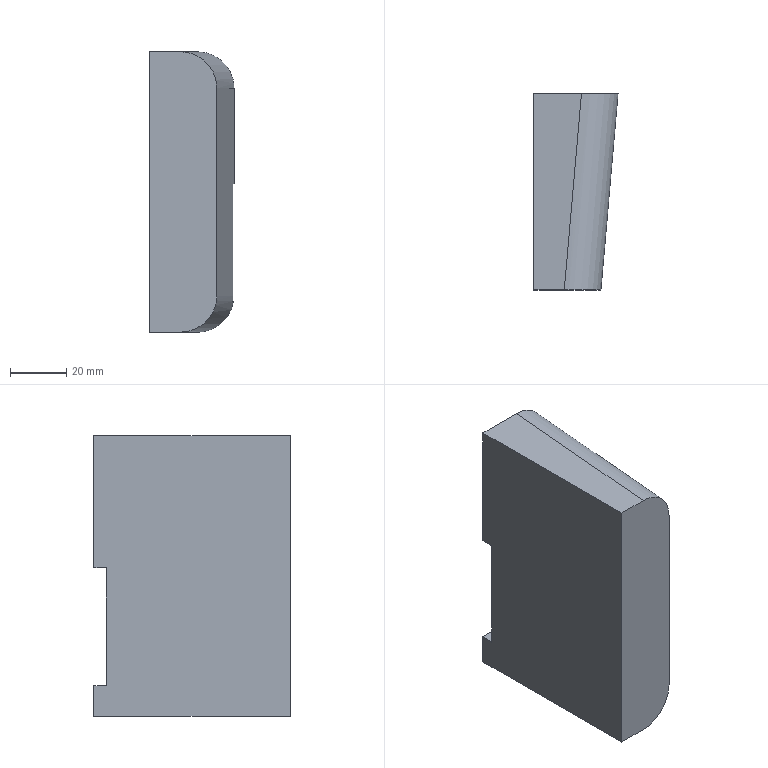Part | STEP file | 1 solid | 12 faces | box 30 x 70 x 100 mm | volume 177836 mm3 | plane 10 | cylinder 2 | commonest cylinder face diameters 26 x2
STEP:
#1=CARTESIAN_POINT('',(0.,0.,0.));
#2=DIRECTION('',(0.,0.,1.));
#3=DIRECTION('',(1.,0.,0.));
#4=AXIS2_PLACEMENT_3D('',#1,#2,#3);
#5=CARTESIAN_POINT('',(37.138,70.,139.451));
#6=VERTEX_POINT('',#5);
#7=CARTESIAN_POINT('',(66.97,70.,139.451));
#8=VERTEX_POINT('',#7);
#9=CARTESIAN_POINT('',(-72.862,70.,139.451));
#10=DIRECTION('',(1.,0.,0.));
#11=VECTOR('',#10,1.);
#12=LINE('',#9,#11);
#13=CARTESIAN_POINT('',(-72.862,70.,-363.47));
#14=DIRECTION('',(0.,-1.,0.));
#15=DIRECTION('',(0.,0.,-1.));
#16=AXIS2_PLACEMENT_3D('',#13,#14,#15);
#17=PLANE('',#16);
#18=CARTESIAN_POINT('',(-502.922,0.));
#19=DIRECTION('',(0.,1.));
#20=VECTOR('',#19,1.);
#21=LINE('',#18,#20);
#22=(GEOMETRIC_REPRESENTATION_CONTEXT(2)PARAMETRIC_REPRESENTATION_CONTEXT()REPRESENTATION_CONTEXT('',''));
#23=DEFINITIONAL_REPRESENTATION('',(#21),#22);
#24=PCURVE('',#17,#23);
#25=CARTESIAN_POINT('',(47.085,69.939,139.451));
#26=DIRECTION('',(0.,0.,1.));
#27=DIRECTION('',(-1.,0.,0.));
#28=AXIS2_PLACEMENT_3D('',#25,#26,#27);
#29=PLANE('',#28);
#30=CARTESIAN_POINT('',(119.948,-0.06099));
#31=DIRECTION('',(-1.,0.));
#32=VECTOR('',#31,1.);
#33=LINE('',#30,#32);
#34=(GEOMETRIC_REPRESENTATION_CONTEXT(2)PARAMETRIC_REPRESENTATION_CONTEXT()REPRESENTATION_CONTEXT('',''));
#35=DEFINITIONAL_REPRESENTATION('',(#33),#34);
#36=PCURVE('',#29,#35);
#37=SURFACE_CURVE('',#12,(#24,#36),.PCURVE_S1.);
#38=EDGE_CURVE('',#6,#8,#37,.T.);
#39=ORIENTED_EDGE('',*,*,#38,.T.);
#40=CARTESIAN_POINT('',(54.088,70.,128.53));
#41=VERTEX_POINT('',#40);
#42=CARTESIAN_POINT('',(66.97,70.,139.451));
#43=CARTESIAN_POINT('',(65.898,70.,132.858));
#44=CARTESIAN_POINT('',(60.792,70.,128.53));
#45=CARTESIAN_POINT('',(54.088,70.,128.53));
#46=(BOUNDED_CURVE()B_SPLINE_CURVE(3,(#42,#43,#44,#45),.UNSPECIFIED.,.F.,.F.)B_SPLINE_CURVE_WITH_KNOTS((4,4),(3.302,4.712),.PIECEWISE_BEZIER_KNOTS.)CURVE()GEOMETRIC_REPRESENTATION_ITEM()RATIONAL_B_SPLINE_CURVE((1.,0.841,0.841,1.))REPRESENTATION_ITEM(''));
#47=CARTESIAN_POINT('',(-502.922,139.832));
#48=CARTESIAN_POINT('',(-496.329,138.76));
#49=CARTESIAN_POINT('',(-492.,133.655));
#50=CARTESIAN_POINT('',(-492.,126.95));
#51=(BOUNDED_CURVE()B_SPLINE_CURVE(3,(#47,#48,#49,#50),.UNSPECIFIED.,.F.,.F.)B_SPLINE_CURVE_WITH_KNOTS((4,4),(3.302,4.712),.PIECEWISE_BEZIER_KNOTS.)CURVE()GEOMETRIC_REPRESENTATION_ITEM()RATIONAL_B_SPLINE_CURVE((1.,0.841,0.841,1.))REPRESENTATION_ITEM(''));
#52=(GEOMETRIC_REPRESENTATION_CONTEXT(2)PARAMETRIC_REPRESENTATION_CONTEXT()REPRESENTATION_CONTEXT('',''));
#53=DEFINITIONAL_REPRESENTATION('',(#51),#52);
#54=PCURVE('',#17,#53);
#55=CARTESIAN_POINT('',(61.057,149.657,141.53));
#56=DIRECTION('',(-0.08716,-0.9962,0.));
#57=DIRECTION('',(0.9962,-0.08716,0.));
#58=AXIS2_PLACEMENT_3D('',#55,#56,#57);
#59=CYLINDRICAL_SURFACE('',#58,13.);
#60=CARTESIAN_POINT('',(6.123,78.839));
#61=CARTESIAN_POINT('',(6.103,78.842));
#62=CARTESIAN_POINT('',(6.063,78.851));
#63=CARTESIAN_POINT('',(6.003,78.868));
#64=CARTESIAN_POINT('',(5.941,78.889));
#65=CARTESIAN_POINT('',(5.878,78.916));
#66=CARTESIAN_POINT('',(5.814,78.946));
#67=CARTESIAN_POINT('',(5.749,78.982));
#68=CARTESIAN_POINT('',(5.684,79.022));
#69=CARTESIAN_POINT('',(5.618,79.066));
#70=CARTESIAN_POINT('',(5.551,79.115));
#71=CARTESIAN_POINT('',(5.484,79.167));
#72=CARTESIAN_POINT('',(5.418,79.224));
#73=CARTESIAN_POINT('',(5.351,79.283));
#74=CARTESIAN_POINT('',(5.284,79.346));
#75=CARTESIAN_POINT('',(5.217,79.411));
#76=CARTESIAN_POINT('',(5.151,79.478));
#77=CARTESIAN_POINT('',(5.086,79.546));
#78=CARTESIAN_POINT('',(5.021,79.615));
#79=CARTESIAN_POINT('',(4.957,79.685));
#80=CARTESIAN_POINT('',(4.894,79.755));
#81=CARTESIAN_POINT('',(4.833,79.825));
#82=CARTESIAN_POINT('',(4.772,79.894));
#83=CARTESIAN_POINT('',(4.732,79.939));
#84=CARTESIAN_POINT('',(4.712,79.961));
#85=B_SPLINE_CURVE_WITH_KNOTS('',3,(#60,#61,#62,#63,#64,#65,#66,#67,#68,#69,#70,#71,#72,#73,#74,#75,#76,#77,#78,#79,#80,#81,#82,#83,#84),.UNSPECIFIED.,.F.,.F.,(4,1,1,1,1,1,1,1,1,1,1,1,1,1,1,1,1,1,1,1,1,1,4),(3.302,3.366,3.43,3.494,3.559,3.623,3.687,3.751,3.815,3.879,3.943,4.007,4.071,4.135,4.2,4.264,4.328,4.392,4.456,4.52,4.584,4.648,4.712),.QUASI_UNIFORM_KNOTS.);
#86=(GEOMETRIC_REPRESENTATION_CONTEXT(2)PARAMETRIC_REPRESENTATION_CONTEXT()REPRESENTATION_CONTEXT('',''));
#87=DEFINITIONAL_REPRESENTATION('',(#85),#86);
#88=PCURVE('',#59,#87);
#89=SURFACE_CURVE('',#46,(#54,#88),.PCURVE_S1.);
#90=EDGE_CURVE('',#8,#41,#89,.T.);
#91=ORIENTED_EDGE('',*,*,#90,.T.);
#92=CARTESIAN_POINT('',(37.138,70.,128.53));
#93=VERTEX_POINT('',#92);
#94=CARTESIAN_POINT('',(57.138,70.,128.53));
#95=DIRECTION('',(-1.,0.,0.));
#96=VECTOR('',#95,1.);
#97=LINE('',#94,#96);
#98=CARTESIAN_POINT('',(-492.,130.));
#99=DIRECTION('',(0.,-1.));
#100=VECTOR('',#99,1.);
#101=LINE('',#98,#100);
#102=(GEOMETRIC_REPRESENTATION_CONTEXT(2)PARAMETRIC_REPRESENTATION_CONTEXT()REPRESENTATION_CONTEXT('',''));
#103=DEFINITIONAL_REPRESENTATION('',(#101),#102);
#104=PCURVE('',#17,#103);
#105=CARTESIAN_POINT('',(57.138,150.,128.53));
#106=DIRECTION('',(0.,0.,1.));
#107=DIRECTION('',(1.,0.,0.));
#108=AXIS2_PLACEMENT_3D('',#105,#106,#107);
#109=PLANE('',#108);
#110=CARTESIAN_POINT('',(0.,-80.));
#111=DIRECTION('',(-1.,0.));
#112=VECTOR('',#111,1.);
#113=LINE('',#110,#112);
#114=(GEOMETRIC_REPRESENTATION_CONTEXT(2)PARAMETRIC_REPRESENTATION_CONTEXT()REPRESENTATION_CONTEXT('',''));
#115=DEFINITIONAL_REPRESENTATION('',(#113),#114);
#116=PCURVE('',#109,#115);
#117=SURFACE_CURVE('',#97,(#104,#116),.PCURVE_S1.);
#118=EDGE_CURVE('',#41,#93,#117,.T.);
#119=ORIENTED_EDGE('',*,*,#118,.T.);
#120=CARTESIAN_POINT('',(37.138,70.,128.53));
#121=DIRECTION('',(0.,0.,1.));
#122=VECTOR('',#121,1.);
#123=LINE('',#120,#122);
#124=CARTESIAN_POINT('',(-492.,110.));
#125=DIRECTION('',(-1.,0.));
#126=VECTOR('',#125,1.);
#127=LINE('',#124,#126);
#128=(GEOMETRIC_REPRESENTATION_CONTEXT(2)PARAMETRIC_REPRESENTATION_CONTEXT()REPRESENTATION_CONTEXT('',''));
#129=DEFINITIONAL_REPRESENTATION('',(#127),#128);
#130=PCURVE('',#17,#129);
#131=CARTESIAN_POINT('',(37.138,150.,128.53));
#132=DIRECTION('',(1.,0.,0.));
#133=DIRECTION('',(0.,0.,-1.));
#134=AXIS2_PLACEMENT_3D('',#131,#132,#133);
#135=PLANE('',#134);
#136=CARTESIAN_POINT('',(0.,-80.));
#137=DIRECTION('',(-1.,0.));
#138=VECTOR('',#137,1.);
#139=LINE('',#136,#138);
#140=(GEOMETRIC_REPRESENTATION_CONTEXT(2)PARAMETRIC_REPRESENTATION_CONTEXT()REPRESENTATION_CONTEXT('',''));
#141=DEFINITIONAL_REPRESENTATION('',(#139),#140);
#142=PCURVE('',#135,#141);
#143=SURFACE_CURVE('',#123,(#130,#142),.PCURVE_S1.);
#144=EDGE_CURVE('',#93,#6,#143,.T.);
#145=ORIENTED_EDGE('',*,*,#144,.T.);
#146=EDGE_LOOP('',(#39,#91,#119,#145));
#147=FACE_BOUND('',#146,.T.);
#148=ADVANCED_FACE('',(#147),#17,.F.);
#149=ORIENTED_EDGE('',*,*,#90,.F.);
#150=CARTESIAN_POINT('',(66.576,65.5,139.451));
#151=VERTEX_POINT('',#150);
#152=CARTESIAN_POINT('',(66.774,67.761,139.451));
#153=DIRECTION('',(-0.08716,-0.9962,0.));
#154=VECTOR('',#153,1.);
#155=LINE('',#152,#154);
#156=CARTESIAN_POINT('',(6.123,81.087));
#157=DIRECTION('',(0.,1.));
#158=VECTOR('',#157,1.);
#159=LINE('',#156,#158);
#160=(GEOMETRIC_REPRESENTATION_CONTEXT(2)PARAMETRIC_REPRESENTATION_CONTEXT()REPRESENTATION_CONTEXT('',''));
#161=DEFINITIONAL_REPRESENTATION('',(#159),#160);
#162=PCURVE('',#59,#161);
#163=CARTESIAN_POINT('',(-19.688,2.178));
#164=DIRECTION('',(0.08716,0.9962));
#165=VECTOR('',#164,1.);
#166=LINE('',#163,#165);
#167=(GEOMETRIC_REPRESENTATION_CONTEXT(2)PARAMETRIC_REPRESENTATION_CONTEXT()REPRESENTATION_CONTEXT('',''));
#168=DEFINITIONAL_REPRESENTATION('',(#166),#167);
#169=PCURVE('',#29,#168);
#170=SURFACE_CURVE('',#155,(#162,#169),.PCURVE_S1.);
#171=EDGE_CURVE('',#8,#151,#170,.T.);
#172=ORIENTED_EDGE('',*,*,#171,.T.);
#173=CARTESIAN_POINT('',(66.744,65.5,141.53));
#174=VERTEX_POINT('',#173);
#175=CARTESIAN_POINT('',(66.576,65.5,139.451));
#176=CARTESIAN_POINT('',(66.688,65.5,140.139));
#177=CARTESIAN_POINT('',(66.744,65.5,140.833));
#178=CARTESIAN_POINT('',(66.744,65.5,141.53));
#179=(BOUNDED_CURVE()B_SPLINE_CURVE(3,(#175,#176,#177,#178),.UNSPECIFIED.,.F.,.F.)B_SPLINE_CURVE_WITH_KNOTS((4,4),(2.981,3.142),.PIECEWISE_BEZIER_KNOTS.)CURVE()GEOMETRIC_REPRESENTATION_ITEM()RATIONAL_B_SPLINE_CURVE((1.,0.9979,0.9979,1.))REPRESENTATION_ITEM(''));
#180=CARTESIAN_POINT('',(6.123,83.356));
#181=CARTESIAN_POINT('',(6.125,83.355));
#182=CARTESIAN_POINT('',(6.13,83.355));
#183=CARTESIAN_POINT('',(6.137,83.353));
#184=CARTESIAN_POINT('',(6.145,83.352));
#185=CARTESIAN_POINT('',(6.152,83.351));
#186=CARTESIAN_POINT('',(6.159,83.35));
#187=CARTESIAN_POINT('',(6.166,83.349));
#188=CARTESIAN_POINT('',(6.174,83.348));
#189=CARTESIAN_POINT('',(6.181,83.347));
#190=CARTESIAN_POINT('',(6.188,83.346));
#191=CARTESIAN_POINT('',(6.196,83.346));
#192=CARTESIAN_POINT('',(6.203,83.345));
#193=CARTESIAN_POINT('',(6.21,83.344));
#194=CARTESIAN_POINT('',(6.218,83.344));
#195=CARTESIAN_POINT('',(6.225,83.343));
#196=CARTESIAN_POINT('',(6.232,83.343));
#197=CARTESIAN_POINT('',(6.239,83.342));
#198=CARTESIAN_POINT('',(6.247,83.342));
#199=CARTESIAN_POINT('',(6.254,83.342));
#200=CARTESIAN_POINT('',(6.261,83.341));
#201=CARTESIAN_POINT('',(6.269,83.341));
#202=CARTESIAN_POINT('',(6.276,83.341));
#203=CARTESIAN_POINT('',(6.281,83.341));
#204=CARTESIAN_POINT('',(6.283,83.341));
#205=B_SPLINE_CURVE_WITH_KNOTS('',3,(#180,#181,#182,#183,#184,#185,#186,#187,#188,#189,#190,#191,#192,#193,#194,#195,#196,#197,#198,#199,#200,#201,#202,#203,#204),.UNSPECIFIED.,.F.,.F.,(4,1,1,1,1,1,1,1,1,1,1,1,1,1,1,1,1,1,1,1,1,1,4),(2.981,2.988,2.996,3.003,3.01,3.018,3.025,3.032,3.039,3.047,3.054,3.061,3.069,3.076,3.083,3.091,3.098,3.105,3.112,3.12,3.127,3.134,3.142),.QUASI_UNIFORM_KNOTS.);
#206=(GEOMETRIC_REPRESENTATION_CONTEXT(2)PARAMETRIC_REPRESENTATION_CONTEXT()REPRESENTATION_CONTEXT('',''));
#207=DEFINITIONAL_REPRESENTATION('',(#205),#206);
#208=PCURVE('',#59,#207);
#209=CARTESIAN_POINT('',(62.138,65.5,160.451));
#210=DIRECTION('',(0.,1.,0.));
#211=DIRECTION('',(0.,0.,1.));
#212=AXIS2_PLACEMENT_3D('',#209,#210,#211);
#213=PLANE('',#212);
#214=CARTESIAN_POINT('',(-21.,4.438));
#215=CARTESIAN_POINT('',(-20.312,4.55));
#216=CARTESIAN_POINT('',(-19.618,4.606));
#217=CARTESIAN_POINT('',(-18.922,4.606));
#218=(BOUNDED_CURVE()B_SPLINE_CURVE(3,(#214,#215,#216,#217),.UNSPECIFIED.,.F.,.F.)B_SPLINE_CURVE_WITH_KNOTS((4,4),(2.981,3.142),.PIECEWISE_BEZIER_KNOTS.)CURVE()GEOMETRIC_REPRESENTATION_ITEM()RATIONAL_B_SPLINE_CURVE((1.,0.9979,0.9979,1.))REPRESENTATION_ITEM(''));
#219=(GEOMETRIC_REPRESENTATION_CONTEXT(2)PARAMETRIC_REPRESENTATION_CONTEXT()REPRESENTATION_CONTEXT('',''));
#220=DEFINITIONAL_REPRESENTATION('',(#218),#219);
#221=PCURVE('',#213,#220);
#222=SURFACE_CURVE('',#179,(#208,#221),.PCURVE_S1.);
#223=EDGE_CURVE('',#151,#174,#222,.T.);
#224=ORIENTED_EDGE('',*,*,#223,.T.);
#225=CARTESIAN_POINT('',(61.013,0.,141.53));
#226=VERTEX_POINT('',#225);
#227=CARTESIAN_POINT('',(67.138,70.,141.53));
#228=DIRECTION('',(0.08716,0.9962,0.));
#229=VECTOR('',#228,1.);
#230=LINE('',#227,#229);
#231=CARTESIAN_POINT('',(6.283,78.824));
#232=DIRECTION('',(0.,-1.));
#233=VECTOR('',#232,1.);
#234=LINE('',#231,#233);
#235=(GEOMETRIC_REPRESENTATION_CONTEXT(2)PARAMETRIC_REPRESENTATION_CONTEXT()REPRESENTATION_CONTEXT('',''));
#236=DEFINITIONAL_REPRESENTATION('',(#234),#235);
#237=PCURVE('',#59,#236);
#238=CARTESIAN_POINT('',(67.138,70.,178.53));
#239=DIRECTION('',(-0.9962,0.08716,0.));
#240=DIRECTION('',(-0.08716,-0.9962,0.));
#241=AXIS2_PLACEMENT_3D('',#238,#239,#240);
#242=PLANE('',#241);
#243=CARTESIAN_POINT('',(0.,-37.));
#244=DIRECTION('',(-1.,0.));
#245=VECTOR('',#244,1.);
#246=LINE('',#243,#245);
#247=(GEOMETRIC_REPRESENTATION_CONTEXT(2)PARAMETRIC_REPRESENTATION_CONTEXT()REPRESENTATION_CONTEXT('',''));
#248=DEFINITIONAL_REPRESENTATION('',(#246),#247);
#249=PCURVE('',#242,#248);
#250=SURFACE_CURVE('',#230,(#237,#249),.PCURVE_S1.);
#251=EDGE_CURVE('',#226,#174,#250,.T.);
#252=ORIENTED_EDGE('',*,*,#251,.F.);
#253=CARTESIAN_POINT('',(47.964,0.,128.53));
#254=VERTEX_POINT('',#253);
#255=CARTESIAN_POINT('',(47.964,0.,128.53));
#256=CARTESIAN_POINT('',(55.608,0.,128.53));
#257=CARTESIAN_POINT('',(61.013,0.,133.914));
#258=CARTESIAN_POINT('',(61.013,0.,141.53));
#259=(BOUNDED_CURVE()B_SPLINE_CURVE(3,(#255,#256,#257,#258),.UNSPECIFIED.,.F.,.F.)B_SPLINE_CURVE_WITH_KNOTS((4,4),(1.571,3.142),.PIECEWISE_BEZIER_KNOTS.)CURVE()GEOMETRIC_REPRESENTATION_ITEM()RATIONAL_B_SPLINE_CURVE((1.,0.8047,0.8047,1.))REPRESENTATION_ITEM(''));
#260=CARTESIAN_POINT('',(4.712,150.229));
#261=CARTESIAN_POINT('',(4.734,150.204));
#262=CARTESIAN_POINT('',(4.777,150.155));
#263=CARTESIAN_POINT('',(4.844,150.079));
#264=CARTESIAN_POINT('',(4.912,150.003));
#265=CARTESIAN_POINT('',(4.982,149.925));
#266=CARTESIAN_POINT('',(5.053,149.848));
#267=CARTESIAN_POINT('',(5.125,149.772));
#268=CARTESIAN_POINT('',(5.199,149.697));
#269=CARTESIAN_POINT('',(5.273,149.624));
#270=CARTESIAN_POINT('',(5.347,149.553));
#271=CARTESIAN_POINT('',(5.422,149.487));
#272=CARTESIAN_POINT('',(5.498,149.424));
#273=CARTESIAN_POINT('',(5.573,149.365));
#274=CARTESIAN_POINT('',(5.648,149.312));
#275=CARTESIAN_POINT('',(5.723,149.264));
#276=CARTESIAN_POINT('',(5.797,149.222));
#277=CARTESIAN_POINT('',(5.87,149.186));
#278=CARTESIAN_POINT('',(5.942,149.156));
#279=CARTESIAN_POINT('',(6.013,149.132));
#280=CARTESIAN_POINT('',(6.083,149.113));
#281=CARTESIAN_POINT('',(6.152,149.1));
#282=CARTESIAN_POINT('',(6.218,149.093));
#283=CARTESIAN_POINT('',(6.262,149.091));
#284=CARTESIAN_POINT('',(6.283,149.091));
#285=B_SPLINE_CURVE_WITH_KNOTS('',3,(#260,#261,#262,#263,#264,#265,#266,#267,#268,#269,#270,#271,#272,#273,#274,#275,#276,#277,#278,#279,#280,#281,#282,#283,#284),.UNSPECIFIED.,.F.,.F.,(4,1,1,1,1,1,1,1,1,1,1,1,1,1,1,1,1,1,1,1,1,1,4),(1.571,1.642,1.714,1.785,1.856,1.928,1.999,2.071,2.142,2.213,2.285,2.356,2.428,2.499,2.57,2.642,2.713,2.785,2.856,2.927,2.999,3.07,3.142),.QUASI_UNIFORM_KNOTS.);
#286=(GEOMETRIC_REPRESENTATION_CONTEXT(2)PARAMETRIC_REPRESENTATION_CONTEXT()REPRESENTATION_CONTEXT('',''));
#287=DEFINITIONAL_REPRESENTATION('',(#285),#286);
#288=PCURVE('',#59,#287);
#289=CARTESIAN_POINT('',(52.138,0.,178.53));
#290=DIRECTION('',(0.,1.,0.));
#291=DIRECTION('',(0.,0.,1.));
#292=AXIS2_PLACEMENT_3D('',#289,#290,#291);
#293=PLANE('',#292);
#294=CARTESIAN_POINT('',(-50.,-4.174));
#295=CARTESIAN_POINT('',(-50.,3.47));
#296=CARTESIAN_POINT('',(-44.615,8.876));
#297=CARTESIAN_POINT('',(-37.,8.876));
#298=(BOUNDED_CURVE()B_SPLINE_CURVE(3,(#294,#295,#296,#297),.UNSPECIFIED.,.F.,.F.)B_SPLINE_CURVE_WITH_KNOTS((4,4),(1.571,3.142),.PIECEWISE_BEZIER_KNOTS.)CURVE()GEOMETRIC_REPRESENTATION_ITEM()RATIONAL_B_SPLINE_CURVE((1.,0.8047,0.8047,1.))REPRESENTATION_ITEM(''));
#299=(GEOMETRIC_REPRESENTATION_CONTEXT(2)PARAMETRIC_REPRESENTATION_CONTEXT()REPRESENTATION_CONTEXT('',''));
#300=DEFINITIONAL_REPRESENTATION('',(#298),#299);
#301=PCURVE('',#293,#300);
#302=SURFACE_CURVE('',#259,(#288,#301),.PCURVE_S1.);
#303=EDGE_CURVE('',#254,#226,#302,.T.);
#304=ORIENTED_EDGE('',*,*,#303,.F.);
#305=CARTESIAN_POINT('',(61.057,149.657,128.53));
#306=DIRECTION('',(-0.08716,-0.9962,0.));
#307=VECTOR('',#306,1.);
#308=LINE('',#305,#307);
#309=CARTESIAN_POINT('',(4.712,0.));
#310=DIRECTION('',(0.,1.));
#311=VECTOR('',#310,1.);
#312=LINE('',#309,#311);
#313=(GEOMETRIC_REPRESENTATION_CONTEXT(2)PARAMETRIC_REPRESENTATION_CONTEXT()REPRESENTATION_CONTEXT('',''));
#314=DEFINITIONAL_REPRESENTATION('',(#312),#313);
#315=PCURVE('',#59,#314);
#316=CARTESIAN_POINT('',(3.919,-0.3429));
#317=DIRECTION('',(-0.08716,-0.9962));
#318=VECTOR('',#317,1.);
#319=LINE('',#316,#318);
#320=(GEOMETRIC_REPRESENTATION_CONTEXT(2)PARAMETRIC_REPRESENTATION_CONTEXT()REPRESENTATION_CONTEXT('',''));
#321=DEFINITIONAL_REPRESENTATION('',(#319),#320);
#322=PCURVE('',#109,#321);
#323=SURFACE_CURVE('',#308,(#315,#322),.PCURVE_S1.);
#324=EDGE_CURVE('',#41,#254,#323,.T.);
#325=ORIENTED_EDGE('',*,*,#324,.F.);
#326=EDGE_LOOP('',(#149,#172,#224,#252,#304,#325));
#327=FACE_BOUND('',#326,.T.);
#328=ADVANCED_FACE('',(#327),#59,.T.);
#329=CARTESIAN_POINT('',(37.138,65.5,181.451));
#330=VERTEX_POINT('',#329);
#331=CARTESIAN_POINT('',(37.138,65.5,139.451));
#332=VERTEX_POINT('',#331);
#333=CARTESIAN_POINT('',(37.138,65.5,108.53));
#334=DIRECTION('',(0.,0.,-1.));
#335=VECTOR('',#334,1.);
#336=LINE('',#333,#335);
#337=CARTESIAN_POINT('',(20.,-84.5));
#338=DIRECTION('',(1.,0.));
#339=VECTOR('',#338,1.);
#340=LINE('',#337,#339);
#341=(GEOMETRIC_REPRESENTATION_CONTEXT(2)PARAMETRIC_REPRESENTATION_CONTEXT()REPRESENTATION_CONTEXT('',''));
#342=DEFINITIONAL_REPRESENTATION('',(#340),#341);
#343=PCURVE('',#135,#342);
#344=CARTESIAN_POINT('',(-51.922,-25.));
#345=DIRECTION('',(-1.,0.));
#346=VECTOR('',#345,1.);
#347=LINE('',#344,#346);
#348=(GEOMETRIC_REPRESENTATION_CONTEXT(2)PARAMETRIC_REPRESENTATION_CONTEXT()REPRESENTATION_CONTEXT('',''));
#349=DEFINITIONAL_REPRESENTATION('',(#347),#348);
#350=PCURVE('',#213,#349);
#351=SURFACE_CURVE('',#336,(#343,#350),.PCURVE_S1.);
#352=EDGE_CURVE('',#330,#332,#351,.T.);
#353=ORIENTED_EDGE('',*,*,#352,.T.);
#354=CARTESIAN_POINT('',(37.138,69.939,139.451));
#355=DIRECTION('',(0.,1.,0.));
#356=VECTOR('',#355,1.);
#357=LINE('',#354,#356);
#358=CARTESIAN_POINT('',(-10.922,-80.061));
#359=DIRECTION('',(0.,1.));
#360=VECTOR('',#359,1.);
#361=LINE('',#358,#360);
#362=(GEOMETRIC_REPRESENTATION_CONTEXT(2)PARAMETRIC_REPRESENTATION_CONTEXT()REPRESENTATION_CONTEXT('',''));
#363=DEFINITIONAL_REPRESENTATION('',(#361),#362);
#364=PCURVE('',#135,#363);
#365=CARTESIAN_POINT('',(9.948,0.));
#366=DIRECTION('',(0.,-1.));
#367=VECTOR('',#366,1.);
#368=LINE('',#365,#367);
#369=(GEOMETRIC_REPRESENTATION_CONTEXT(2)PARAMETRIC_REPRESENTATION_CONTEXT()REPRESENTATION_CONTEXT('',''));
#370=DEFINITIONAL_REPRESENTATION('',(#368),#369);
#371=PCURVE('',#29,#370);
#372=SURFACE_CURVE('',#357,(#364,#371),.PCURVE_S1.);
#373=EDGE_CURVE('',#332,#6,#372,.T.);
#374=ORIENTED_EDGE('',*,*,#373,.T.);
#375=ORIENTED_EDGE('',*,*,#144,.F.);
#376=CARTESIAN_POINT('',(37.138,0.,128.53));
#377=VERTEX_POINT('',#376);
#378=CARTESIAN_POINT('',(37.138,150.,128.53));
#379=DIRECTION('',(0.,-1.,0.));
#380=VECTOR('',#379,1.);
#381=LINE('',#378,#380);
#382=CARTESIAN_POINT('',(0.,0.));
#383=DIRECTION('',(0.,-1.));
#384=VECTOR('',#383,1.);
#385=LINE('',#382,#384);
#386=(GEOMETRIC_REPRESENTATION_CONTEXT(2)PARAMETRIC_REPRESENTATION_CONTEXT()REPRESENTATION_CONTEXT('',''));
#387=DEFINITIONAL_REPRESENTATION('',(#385),#386);
#388=PCURVE('',#135,#387);
#389=CARTESIAN_POINT('',(-20.,0.));
#390=DIRECTION('',(0.,-1.));
#391=VECTOR('',#390,1.);
#392=LINE('',#389,#391);
#393=(GEOMETRIC_REPRESENTATION_CONTEXT(2)PARAMETRIC_REPRESENTATION_CONTEXT()REPRESENTATION_CONTEXT('',''));
#394=DEFINITIONAL_REPRESENTATION('',(#392),#393);
#395=PCURVE('',#109,#394);
#396=SURFACE_CURVE('',#381,(#388,#395),.PCURVE_S1.);
#397=EDGE_CURVE('',#93,#377,#396,.T.);
#398=ORIENTED_EDGE('',*,*,#397,.T.);
#399=CARTESIAN_POINT('',(37.138,0.,228.53));
#400=VERTEX_POINT('',#399);
#401=CARTESIAN_POINT('',(37.138,0.,128.53));
#402=DIRECTION('',(0.,0.,1.));
#403=VECTOR('',#402,1.);
#404=LINE('',#401,#403);
#405=CARTESIAN_POINT('',(0.,-150.));
#406=DIRECTION('',(-1.,0.));
#407=VECTOR('',#406,1.);
#408=LINE('',#405,#407);
#409=(GEOMETRIC_REPRESENTATION_CONTEXT(2)PARAMETRIC_REPRESENTATION_CONTEXT()REPRESENTATION_CONTEXT('',''));
#410=DEFINITIONAL_REPRESENTATION('',(#408),#409);
#411=PCURVE('',#135,#410);
#412=CARTESIAN_POINT('',(-50.,-15.));
#413=DIRECTION('',(1.,0.));
#414=VECTOR('',#413,1.);
#415=LINE('',#412,#414);
#416=(GEOMETRIC_REPRESENTATION_CONTEXT(2)PARAMETRIC_REPRESENTATION_CONTEXT()REPRESENTATION_CONTEXT('',''));
#417=DEFINITIONAL_REPRESENTATION('',(#415),#416);
#418=PCURVE('',#293,#417);
#419=SURFACE_CURVE('',#404,(#411,#418),.PCURVE_S1.);
#420=EDGE_CURVE('',#377,#400,#419,.T.);
#421=ORIENTED_EDGE('',*,*,#420,.T.);
#422=CARTESIAN_POINT('',(37.138,70.,228.53));
#423=VERTEX_POINT('',#422);
#424=CARTESIAN_POINT('',(37.138,150.,228.53));
#425=DIRECTION('',(0.,-1.,0.));
#426=VECTOR('',#425,1.);
#427=LINE('',#424,#426);
#428=CARTESIAN_POINT('',(-100.,0.));
#429=DIRECTION('',(0.,-1.));
#430=VECTOR('',#429,1.);
#431=LINE('',#428,#430);
#432=(GEOMETRIC_REPRESENTATION_CONTEXT(2)PARAMETRIC_REPRESENTATION_CONTEXT()REPRESENTATION_CONTEXT('',''));
#433=DEFINITIONAL_REPRESENTATION('',(#431),#432);
#434=PCURVE('',#135,#433);
#435=CARTESIAN_POINT('',(37.138,150.,228.53));
#436=DIRECTION('',(0.,0.,-1.));
#437=DIRECTION('',(-1.,0.,0.));
#438=AXIS2_PLACEMENT_3D('',#435,#436,#437);
#439=PLANE('',#438);
#440=CARTESIAN_POINT('',(0.,0.));
#441=DIRECTION('',(0.,-1.));
#442=VECTOR('',#441,1.);
#443=LINE('',#440,#442);
#444=(GEOMETRIC_REPRESENTATION_CONTEXT(2)PARAMETRIC_REPRESENTATION_CONTEXT()REPRESENTATION_CONTEXT('',''));
#445=DEFINITIONAL_REPRESENTATION('',(#443),#444);
#446=PCURVE('',#439,#445);
#447=SURFACE_CURVE('',#427,(#434,#446),.PCURVE_S1.);
#448=EDGE_CURVE('',#423,#400,#447,.T.);
#449=ORIENTED_EDGE('',*,*,#448,.F.);
#450=CARTESIAN_POINT('',(37.138,70.,181.451));
#451=VERTEX_POINT('',#450);
#452=CARTESIAN_POINT('',(37.138,70.,128.53));
#453=DIRECTION('',(0.,0.,1.));
#454=VECTOR('',#453,1.);
#455=LINE('',#452,#454);
#456=CARTESIAN_POINT('',(0.,-80.));
#457=DIRECTION('',(-1.,0.));
#458=VECTOR('',#457,1.);
#459=LINE('',#456,#458);
#460=(GEOMETRIC_REPRESENTATION_CONTEXT(2)PARAMETRIC_REPRESENTATION_CONTEXT()REPRESENTATION_CONTEXT('',''));
#461=DEFINITIONAL_REPRESENTATION('',(#459),#460);
#462=PCURVE('',#135,#461);
#463=CARTESIAN_POINT('',(-72.862,70.,-363.47));
#464=DIRECTION('',(0.,-1.,0.));
#465=DIRECTION('',(0.,0.,-1.));
#466=AXIS2_PLACEMENT_3D('',#463,#464,#465);
#467=PLANE('',#466);
#468=CARTESIAN_POINT('',(-492.,110.));
#469=DIRECTION('',(-1.,0.));
#470=VECTOR('',#469,1.);
#471=LINE('',#468,#470);
#472=(GEOMETRIC_REPRESENTATION_CONTEXT(2)PARAMETRIC_REPRESENTATION_CONTEXT()REPRESENTATION_CONTEXT('',''));
#473=DEFINITIONAL_REPRESENTATION('',(#471),#472);
#474=PCURVE('',#467,#473);
#475=SURFACE_CURVE('',#455,(#462,#474),.PCURVE_S1.);
#476=EDGE_CURVE('',#451,#423,#475,.T.);
#477=ORIENTED_EDGE('',*,*,#476,.F.);
#478=CARTESIAN_POINT('',(37.138,69.939,181.451));
#479=DIRECTION('',(0.,1.,0.));
#480=VECTOR('',#479,1.);
#481=LINE('',#478,#480);
#482=CARTESIAN_POINT('',(-52.922,-80.061));
#483=DIRECTION('',(0.,1.));
#484=VECTOR('',#483,1.);
#485=LINE('',#482,#484);
#486=(GEOMETRIC_REPRESENTATION_CONTEXT(2)PARAMETRIC_REPRESENTATION_CONTEXT()REPRESENTATION_CONTEXT('',''));
#487=DEFINITIONAL_REPRESENTATION('',(#485),#486);
#488=PCURVE('',#135,#487);
#489=CARTESIAN_POINT('',(47.085,69.939,181.451));
#490=DIRECTION('',(0.,0.,1.));
#491=DIRECTION('',(-1.,0.,0.));
#492=AXIS2_PLACEMENT_3D('',#489,#490,#491);
#493=PLANE('',#492);
#494=CARTESIAN_POINT('',(9.948,0.));
#495=DIRECTION('',(0.,-1.));
#496=VECTOR('',#495,1.);
#497=LINE('',#494,#496);
#498=(GEOMETRIC_REPRESENTATION_CONTEXT(2)PARAMETRIC_REPRESENTATION_CONTEXT()REPRESENTATION_CONTEXT('',''));
#499=DEFINITIONAL_REPRESENTATION('',(#497),#498);
#500=PCURVE('',#493,#499);
#501=SURFACE_CURVE('',#481,(#488,#500),.PCURVE_S1.);
#502=EDGE_CURVE('',#330,#451,#501,.T.);
#503=ORIENTED_EDGE('',*,*,#502,.F.);
#504=EDGE_LOOP('',(#353,#374,#375,#398,#421,#449,#477,#503));
#505=FACE_BOUND('',#504,.T.);
#506=ADVANCED_FACE('',(#505),#135,.F.);
#507=CARTESIAN_POINT('',(67.138,70.,215.53));
#508=VERTEX_POINT('',#507);
#509=CARTESIAN_POINT('',(67.138,70.,181.451));
#510=VERTEX_POINT('',#509);
#511=CARTESIAN_POINT('',(67.138,70.,178.53));
#512=DIRECTION('',(0.,0.,-1.));
#513=VECTOR('',#512,1.);
#514=LINE('',#511,#513);
#515=CARTESIAN_POINT('',(-542.,140.));
#516=DIRECTION('',(1.,0.));
#517=VECTOR('',#516,1.);
#518=LINE('',#515,#517);
#519=(GEOMETRIC_REPRESENTATION_CONTEXT(2)PARAMETRIC_REPRESENTATION_CONTEXT()REPRESENTATION_CONTEXT('',''));
#520=DEFINITIONAL_REPRESENTATION('',(#518),#519);
#521=PCURVE('',#467,#520);
#522=CARTESIAN_POINT('',(0.,0.));
#523=DIRECTION('',(0.,-1.));
#524=VECTOR('',#523,1.);
#525=LINE('',#522,#524);
#526=(GEOMETRIC_REPRESENTATION_CONTEXT(2)PARAMETRIC_REPRESENTATION_CONTEXT()REPRESENTATION_CONTEXT('',''));
#527=DEFINITIONAL_REPRESENTATION('',(#525),#526);
#528=PCURVE('',#242,#527);
#529=SURFACE_CURVE('',#514,(#521,#528),.PCURVE_S1.);
#530=EDGE_CURVE('',#508,#510,#529,.T.);
#531=ORIENTED_EDGE('',*,*,#530,.T.);
#532=CARTESIAN_POINT('',(-72.862,70.,181.451));
#533=DIRECTION('',(1.,0.,0.));
#534=VECTOR('',#533,1.);
#535=LINE('',#532,#534);
#536=CARTESIAN_POINT('',(-544.922,0.));
#537=DIRECTION('',(0.,1.));
#538=VECTOR('',#537,1.);
#539=LINE('',#536,#538);
#540=(GEOMETRIC_REPRESENTATION_CONTEXT(2)PARAMETRIC_REPRESENTATION_CONTEXT()REPRESENTATION_CONTEXT('',''));
#541=DEFINITIONAL_REPRESENTATION('',(#539),#540);
#542=PCURVE('',#467,#541);
#543=CARTESIAN_POINT('',(119.948,-0.06099));
#544=DIRECTION('',(-1.,0.));
#545=VECTOR('',#544,1.);
#546=LINE('',#543,#545);
#547=(GEOMETRIC_REPRESENTATION_CONTEXT(2)PARAMETRIC_REPRESENTATION_CONTEXT()REPRESENTATION_CONTEXT('',''));
#548=DEFINITIONAL_REPRESENTATION('',(#546),#547);
#549=PCURVE('',#493,#548);
#550=SURFACE_CURVE('',#535,(#542,#549),.PCURVE_S1.);
#551=EDGE_CURVE('',#451,#510,#550,.T.);
#552=ORIENTED_EDGE('',*,*,#551,.F.);
#553=ORIENTED_EDGE('',*,*,#476,.T.);
#554=CARTESIAN_POINT('',(54.088,70.,228.53));
#555=VERTEX_POINT('',#554);
#556=CARTESIAN_POINT('',(37.138,70.,228.53));
#557=DIRECTION('',(1.,0.,0.));
#558=VECTOR('',#557,1.);
#559=LINE('',#556,#558);
#560=CARTESIAN_POINT('',(-592.,110.));
#561=DIRECTION('',(0.,1.));
#562=VECTOR('',#561,1.);
#563=LINE('',#560,#562);
#564=(GEOMETRIC_REPRESENTATION_CONTEXT(2)PARAMETRIC_REPRESENTATION_CONTEXT()REPRESENTATION_CONTEXT('',''));
#565=DEFINITIONAL_REPRESENTATION('',(#563),#564);
#566=PCURVE('',#467,#565);
#567=CARTESIAN_POINT('',(0.,-80.));
#568=DIRECTION('',(-1.,0.));
#569=VECTOR('',#568,1.);
#570=LINE('',#567,#569);
#571=(GEOMETRIC_REPRESENTATION_CONTEXT(2)PARAMETRIC_REPRESENTATION_CONTEXT()REPRESENTATION_CONTEXT('',''));
#572=DEFINITIONAL_REPRESENTATION('',(#570),#571);
#573=PCURVE('',#439,#572);
#574=SURFACE_CURVE('',#559,(#566,#573),.PCURVE_S1.);
#575=EDGE_CURVE('',#423,#555,#574,.T.);
#576=ORIENTED_EDGE('',*,*,#575,.T.);
#577=CARTESIAN_POINT('',(54.088,70.,228.53));
#578=CARTESIAN_POINT('',(61.732,70.,228.53));
#579=CARTESIAN_POINT('',(67.138,70.,223.145));
#580=CARTESIAN_POINT('',(67.138,70.,215.53));
#581=(BOUNDED_CURVE()B_SPLINE_CURVE(3,(#577,#578,#579,#580),.UNSPECIFIED.,.F.,.F.)B_SPLINE_CURVE_WITH_KNOTS((4,4),(1.571,3.142),.PIECEWISE_BEZIER_KNOTS.)CURVE()GEOMETRIC_REPRESENTATION_ITEM()RATIONAL_B_SPLINE_CURVE((1.,0.8047,0.8047,1.))REPRESENTATION_ITEM(''));
#582=CARTESIAN_POINT('',(-592.,126.95));
#583=CARTESIAN_POINT('',(-592.,134.595));
#584=CARTESIAN_POINT('',(-586.615,140.));
#585=CARTESIAN_POINT('',(-579.,140.));
#586=(BOUNDED_CURVE()B_SPLINE_CURVE(3,(#582,#583,#584,#585),.UNSPECIFIED.,.F.,.F.)B_SPLINE_CURVE_WITH_KNOTS((4,4),(1.571,3.142),.PIECEWISE_BEZIER_KNOTS.)CURVE()GEOMETRIC_REPRESENTATION_ITEM()RATIONAL_B_SPLINE_CURVE((1.,0.8047,0.8047,1.))REPRESENTATION_ITEM(''));
#587=(GEOMETRIC_REPRESENTATION_CONTEXT(2)PARAMETRIC_REPRESENTATION_CONTEXT()REPRESENTATION_CONTEXT('',''));
#588=DEFINITIONAL_REPRESENTATION('',(#586),#587);
#589=PCURVE('',#467,#588);
#590=CARTESIAN_POINT('',(54.187,71.133,215.53));
#591=DIRECTION('',(-0.08716,-0.9962,0.));
#592=DIRECTION('',(0.9962,-0.08716,0.));
#593=AXIS2_PLACEMENT_3D('',#590,#591,#592);
#594=CYLINDRICAL_SURFACE('',#593,13.);
#595=CARTESIAN_POINT('',(1.571,1.137));
#596=CARTESIAN_POINT('',(1.549,1.113));
#597=CARTESIAN_POINT('',(1.506,1.064));
#598=CARTESIAN_POINT('',(1.439,0.988));
#599=CARTESIAN_POINT('',(1.371,0.9113));
#600=CARTESIAN_POINT('',(1.301,0.834));
#601=CARTESIAN_POINT('',(1.23,0.7569));
#602=CARTESIAN_POINT('',(1.158,0.6804));
#603=CARTESIAN_POINT('',(1.085,0.6054));
#604=CARTESIAN_POINT('',(1.01,0.5323));
#605=CARTESIAN_POINT('',(0.9358,0.4621));
#606=CARTESIAN_POINT('',(0.8607,0.3952));
#607=CARTESIAN_POINT('',(0.7854,0.3324));
#608=CARTESIAN_POINT('',(0.7101,0.2741));
#609=CARTESIAN_POINT('',(0.635,0.2208));
#610=CARTESIAN_POINT('',(0.5603,0.173));
#611=CARTESIAN_POINT('',(0.4863,0.1309));
#612=CARTESIAN_POINT('',(0.413,0.09472));
#613=CARTESIAN_POINT('',(0.3408,0.06449));
#614=CARTESIAN_POINT('',(0.2697,0.04021));
#615=CARTESIAN_POINT('',(0.2,0.02178));
#616=CARTESIAN_POINT('',(0.1316,0.008981));
#617=CARTESIAN_POINT('',(0.06485,0.001569));
#618=CARTESIAN_POINT('',(0.02143,-0.000003694));
#619=CARTESIAN_POINT('',(0.,0.));
#620=B_SPLINE_CURVE_WITH_KNOTS('',3,(#595,#596,#597,#598,#599,#600,#601,#602,#603,#604,#605,#606,#607,#608,#609,#610,#611,#612,#613,#614,#615,#616,#617,#618,#619),.UNSPECIFIED.,.F.,.F.,(4,1,1,1,1,1,1,1,1,1,1,1,1,1,1,1,1,1,1,1,1,1,4),(1.571,1.642,1.714,1.785,1.856,1.928,1.999,2.071,2.142,2.213,2.285,2.356,2.428,2.499,2.57,2.642,2.713,2.785,2.856,2.927,2.999,3.07,3.142),.QUASI_UNIFORM_KNOTS.);
#621=(GEOMETRIC_REPRESENTATION_CONTEXT(2)PARAMETRIC_REPRESENTATION_CONTEXT()REPRESENTATION_CONTEXT('',''));
#622=DEFINITIONAL_REPRESENTATION('',(#620),#621);
#623=PCURVE('',#594,#622);
#624=SURFACE_CURVE('',#581,(#589,#623),.PCURVE_S1.);
#625=EDGE_CURVE('',#555,#508,#624,.T.);
#626=ORIENTED_EDGE('',*,*,#625,.T.);
#627=EDGE_LOOP('',(#531,#552,#553,#576,#626));
#628=FACE_BOUND('',#627,.T.);
#629=ADVANCED_FACE('',(#628),#467,.F.);
#630=ORIENTED_EDGE('',*,*,#118,.F.);
#631=ORIENTED_EDGE('',*,*,#324,.T.);
#632=CARTESIAN_POINT('',(57.138,0.,128.53));
#633=DIRECTION('',(-1.,0.,0.));
#634=VECTOR('',#633,1.);
#635=LINE('',#632,#634);
#636=CARTESIAN_POINT('',(0.,-150.));
#637=DIRECTION('',(-1.,0.));
#638=VECTOR('',#637,1.);
#639=LINE('',#636,#638);
#640=(GEOMETRIC_REPRESENTATION_CONTEXT(2)PARAMETRIC_REPRESENTATION_CONTEXT()REPRESENTATION_CONTEXT('',''));
#641=DEFINITIONAL_REPRESENTATION('',(#639),#640);
#642=PCURVE('',#109,#641);
#643=CARTESIAN_POINT('',(-50.,5.));
#644=DIRECTION('',(0.,-1.));
#645=VECTOR('',#644,1.);
#646=LINE('',#643,#645);
#647=(GEOMETRIC_REPRESENTATION_CONTEXT(2)PARAMETRIC_REPRESENTATION_CONTEXT()REPRESENTATION_CONTEXT('',''));
#648=DEFINITIONAL_REPRESENTATION('',(#646),#647);
#649=PCURVE('',#293,#648);
#650=SURFACE_CURVE('',#635,(#642,#649),.PCURVE_S1.);
#651=EDGE_CURVE('',#254,#377,#650,.T.);
#652=ORIENTED_EDGE('',*,*,#651,.T.);
#653=ORIENTED_EDGE('',*,*,#397,.F.);
#654=EDGE_LOOP('',(#630,#631,#652,#653));
#655=FACE_BOUND('',#654,.T.);
#656=ADVANCED_FACE('',(#655),#109,.F.);
#657=CARTESIAN_POINT('',(66.744,65.5,181.451));
#658=VERTEX_POINT('',#657);
#659=CARTESIAN_POINT('',(66.744,65.5,178.53));
#660=DIRECTION('',(0.,0.,-1.));
#661=VECTOR('',#660,1.);
#662=LINE('',#659,#661);
#663=CARTESIAN_POINT('',(4.517,0.));
#664=DIRECTION('',(0.,-1.));
#665=VECTOR('',#664,1.);
#666=LINE('',#663,#665);
#667=(GEOMETRIC_REPRESENTATION_CONTEXT(2)PARAMETRIC_REPRESENTATION_CONTEXT()REPRESENTATION_CONTEXT('',''));
#668=DEFINITIONAL_REPRESENTATION('',(#666),#667);
#669=PCURVE('',#242,#668);
#670=CARTESIAN_POINT('',(18.078,4.606));
#671=DIRECTION('',(-1.,0.));
#672=VECTOR('',#671,1.);
#673=LINE('',#670,#672);
#674=(GEOMETRIC_REPRESENTATION_CONTEXT(2)PARAMETRIC_REPRESENTATION_CONTEXT()REPRESENTATION_CONTEXT('',''));
#675=DEFINITIONAL_REPRESENTATION('',(#673),#674);
#676=PCURVE('',#213,#675);
#677=SURFACE_CURVE('',#662,(#669,#676),.PCURVE_S1.);
#678=EDGE_CURVE('',#658,#174,#677,.T.);
#679=ORIENTED_EDGE('',*,*,#678,.F.);
#680=CARTESIAN_POINT('',(67.138,70.,181.451));
#681=DIRECTION('',(0.08716,0.9962,0.));
#682=VECTOR('',#681,1.);
#683=LINE('',#680,#682);
#684=CARTESIAN_POINT('',(0.,2.922));
#685=DIRECTION('',(-1.,0.));
#686=VECTOR('',#685,1.);
#687=LINE('',#684,#686);
#688=(GEOMETRIC_REPRESENTATION_CONTEXT(2)PARAMETRIC_REPRESENTATION_CONTEXT()REPRESENTATION_CONTEXT('',''));
#689=DEFINITIONAL_REPRESENTATION('',(#687),#688);
#690=PCURVE('',#242,#689);
#691=CARTESIAN_POINT('',(-20.052,-0.06099));
#692=DIRECTION('',(-0.08716,-0.9962));
#693=VECTOR('',#692,1.);
#694=LINE('',#691,#693);
#695=(GEOMETRIC_REPRESENTATION_CONTEXT(2)PARAMETRIC_REPRESENTATION_CONTEXT()REPRESENTATION_CONTEXT('',''));
#696=DEFINITIONAL_REPRESENTATION('',(#694),#695);
#697=PCURVE('',#493,#696);
#698=SURFACE_CURVE('',#683,(#690,#697),.PCURVE_S1.);
#699=EDGE_CURVE('',#658,#510,#698,.T.);
#700=ORIENTED_EDGE('',*,*,#699,.T.);
#701=ORIENTED_EDGE('',*,*,#530,.F.);
#702=CARTESIAN_POINT('',(61.013,0.,215.53));
#703=VERTEX_POINT('',#702);
#704=CARTESIAN_POINT('',(67.138,70.,215.53));
#705=DIRECTION('',(-0.08716,-0.9962,0.));
#706=VECTOR('',#705,1.);
#707=LINE('',#704,#706);
#708=CARTESIAN_POINT('',(0.,37.));
#709=DIRECTION('',(1.,0.));
#710=VECTOR('',#709,1.);
#711=LINE('',#708,#710);
#712=(GEOMETRIC_REPRESENTATION_CONTEXT(2)PARAMETRIC_REPRESENTATION_CONTEXT()REPRESENTATION_CONTEXT('',''));
#713=DEFINITIONAL_REPRESENTATION('',(#711),#712);
#714=PCURVE('',#242,#713);
#715=CARTESIAN_POINT('',(0.,0.));
#716=DIRECTION('',(0.,1.));
#717=VECTOR('',#716,1.);
#718=LINE('',#715,#717);
#719=(GEOMETRIC_REPRESENTATION_CONTEXT(2)PARAMETRIC_REPRESENTATION_CONTEXT()REPRESENTATION_CONTEXT('',''));
#720=DEFINITIONAL_REPRESENTATION('',(#718),#719);
#721=PCURVE('',#594,#720);
#722=SURFACE_CURVE('',#707,(#714,#721),.PCURVE_S1.);
#723=EDGE_CURVE('',#508,#703,#722,.T.);
#724=ORIENTED_EDGE('',*,*,#723,.T.);
#725=CARTESIAN_POINT('',(61.013,0.,178.53));
#726=DIRECTION('',(0.,0.,-1.));
#727=VECTOR('',#726,1.);
#728=LINE('',#725,#727);
#729=CARTESIAN_POINT('',(70.267,0.));
#730=DIRECTION('',(0.,-1.));
#731=VECTOR('',#730,1.);
#732=LINE('',#729,#731);
#733=(GEOMETRIC_REPRESENTATION_CONTEXT(2)PARAMETRIC_REPRESENTATION_CONTEXT()REPRESENTATION_CONTEXT('',''));
#734=DEFINITIONAL_REPRESENTATION('',(#732),#733);
#735=PCURVE('',#242,#734);
#736=CARTESIAN_POINT('',(0.,8.876));
#737=DIRECTION('',(-1.,0.));
#738=VECTOR('',#737,1.);
#739=LINE('',#736,#738);
#740=(GEOMETRIC_REPRESENTATION_CONTEXT(2)PARAMETRIC_REPRESENTATION_CONTEXT()REPRESENTATION_CONTEXT('',''));
#741=DEFINITIONAL_REPRESENTATION('',(#739),#740);
#742=PCURVE('',#293,#741);
#743=SURFACE_CURVE('',#728,(#735,#742),.PCURVE_S1.);
#744=EDGE_CURVE('',#703,#226,#743,.T.);
#745=ORIENTED_EDGE('',*,*,#744,.T.);
#746=ORIENTED_EDGE('',*,*,#251,.T.);
#747=EDGE_LOOP('',(#679,#700,#701,#724,#745,#746));
#748=FACE_BOUND('',#747,.T.);
#749=ADVANCED_FACE('',(#748),#242,.F.);
#750=CARTESIAN_POINT('',(47.964,0.,228.53));
#751=VERTEX_POINT('',#750);
#752=CARTESIAN_POINT('',(37.138,0.,228.53));
#753=DIRECTION('',(1.,0.,0.));
#754=VECTOR('',#753,1.);
#755=LINE('',#752,#754);
#756=CARTESIAN_POINT('',(0.,-150.));
#757=DIRECTION('',(-1.,0.));
#758=VECTOR('',#757,1.);
#759=LINE('',#756,#758);
#760=(GEOMETRIC_REPRESENTATION_CONTEXT(2)PARAMETRIC_REPRESENTATION_CONTEXT()REPRESENTATION_CONTEXT('',''));
#761=DEFINITIONAL_REPRESENTATION('',(#759),#760);
#762=PCURVE('',#439,#761);
#763=CARTESIAN_POINT('',(50.,-15.));
#764=DIRECTION('',(0.,1.));
#765=VECTOR('',#764,1.);
#766=LINE('',#763,#765);
#767=(GEOMETRIC_REPRESENTATION_CONTEXT(2)PARAMETRIC_REPRESENTATION_CONTEXT()REPRESENTATION_CONTEXT('',''));
#768=DEFINITIONAL_REPRESENTATION('',(#766),#767);
#769=PCURVE('',#293,#768);
#770=SURFACE_CURVE('',#755,(#762,#769),.PCURVE_S1.);
#771=EDGE_CURVE('',#400,#751,#770,.T.);
#772=ORIENTED_EDGE('',*,*,#771,.T.);
#773=CARTESIAN_POINT('',(60.905,147.921,228.53));
#774=DIRECTION('',(0.08716,0.9962,0.));
#775=VECTOR('',#774,1.);
#776=LINE('',#773,#775);
#777=CARTESIAN_POINT('',(-23.768,-2.079));
#778=DIRECTION('',(-0.08716,0.9962));
#779=VECTOR('',#778,1.);
#780=LINE('',#777,#779);
#781=(GEOMETRIC_REPRESENTATION_CONTEXT(2)PARAMETRIC_REPRESENTATION_CONTEXT()REPRESENTATION_CONTEXT('',''));
#782=DEFINITIONAL_REPRESENTATION('',(#780),#781);
#783=PCURVE('',#439,#782);
#784=CARTESIAN_POINT('',(1.571,-77.081));
#785=DIRECTION('',(0.,-1.));
#786=VECTOR('',#785,1.);
#787=LINE('',#784,#786);
#788=(GEOMETRIC_REPRESENTATION_CONTEXT(2)PARAMETRIC_REPRESENTATION_CONTEXT()REPRESENTATION_CONTEXT('',''));
#789=DEFINITIONAL_REPRESENTATION('',(#787),#788);
#790=PCURVE('',#594,#789);
#791=SURFACE_CURVE('',#776,(#783,#790),.PCURVE_S1.);
#792=EDGE_CURVE('',#751,#555,#791,.T.);
#793=ORIENTED_EDGE('',*,*,#792,.T.);
#794=ORIENTED_EDGE('',*,*,#575,.F.);
#795=ORIENTED_EDGE('',*,*,#448,.T.);
#796=EDGE_LOOP('',(#772,#793,#794,#795));
#797=FACE_BOUND('',#796,.T.);
#798=ADVANCED_FACE('',(#797),#439,.F.);
#799=ORIENTED_EDGE('',*,*,#744,.F.);
#800=CARTESIAN_POINT('',(61.013,0.,215.53));
#801=CARTESIAN_POINT('',(61.013,0.,223.145));
#802=CARTESIAN_POINT('',(55.608,0.,228.53));
#803=CARTESIAN_POINT('',(47.964,0.,228.53));
#804=(BOUNDED_CURVE()B_SPLINE_CURVE(3,(#800,#801,#802,#803),.UNSPECIFIED.,.F.,.F.)B_SPLINE_CURVE_WITH_KNOTS((4,4),(3.142,4.712),.PIECEWISE_BEZIER_KNOTS.)CURVE()GEOMETRIC_REPRESENTATION_ITEM()RATIONAL_B_SPLINE_CURVE((1.,0.8047,0.8047,1.))REPRESENTATION_ITEM(''));
#805=CARTESIAN_POINT('',(37.,8.876));
#806=CARTESIAN_POINT('',(44.615,8.876));
#807=CARTESIAN_POINT('',(50.,3.47));
#808=CARTESIAN_POINT('',(50.,-4.174));
#809=(BOUNDED_CURVE()B_SPLINE_CURVE(3,(#805,#806,#807,#808),.UNSPECIFIED.,.F.,.F.)B_SPLINE_CURVE_WITH_KNOTS((4,4),(3.142,4.712),.PIECEWISE_BEZIER_KNOTS.)CURVE()GEOMETRIC_REPRESENTATION_ITEM()RATIONAL_B_SPLINE_CURVE((1.,0.8047,0.8047,1.))REPRESENTATION_ITEM(''));
#810=(GEOMETRIC_REPRESENTATION_CONTEXT(2)PARAMETRIC_REPRESENTATION_CONTEXT()REPRESENTATION_CONTEXT('',''));
#811=DEFINITIONAL_REPRESENTATION('',(#809),#810);
#812=PCURVE('',#293,#811);
#813=CARTESIAN_POINT('',(0.,70.267));
#814=CARTESIAN_POINT('',(0.02143,70.267));
#815=CARTESIAN_POINT('',(0.06485,70.269));
#816=CARTESIAN_POINT('',(0.1316,70.276));
#817=CARTESIAN_POINT('',(0.2,70.289));
#818=CARTESIAN_POINT('',(0.2697,70.308));
#819=CARTESIAN_POINT('',(0.3408,70.332));
#820=CARTESIAN_POINT('',(0.413,70.362));
#821=CARTESIAN_POINT('',(0.4863,70.398));
#822=CARTESIAN_POINT('',(0.5603,70.44));
#823=CARTESIAN_POINT('',(0.635,70.488));
#824=CARTESIAN_POINT('',(0.7101,70.541));
#825=CARTESIAN_POINT('',(0.7854,70.6));
#826=CARTESIAN_POINT('',(0.8607,70.663));
#827=CARTESIAN_POINT('',(0.9358,70.729));
#828=CARTESIAN_POINT('',(1.01,70.8));
#829=CARTESIAN_POINT('',(1.085,70.873));
#830=CARTESIAN_POINT('',(1.158,70.948));
#831=CARTESIAN_POINT('',(1.23,71.024));
#832=CARTESIAN_POINT('',(1.301,71.101));
#833=CARTESIAN_POINT('',(1.371,71.179));
#834=CARTESIAN_POINT('',(1.439,71.255));
#835=CARTESIAN_POINT('',(1.506,71.331));
#836=CARTESIAN_POINT('',(1.549,71.38));
#837=CARTESIAN_POINT('',(1.571,71.405));
#838=B_SPLINE_CURVE_WITH_KNOTS('',3,(#813,#814,#815,#816,#817,#818,#819,#820,#821,#822,#823,#824,#825,#826,#827,#828,#829,#830,#831,#832,#833,#834,#835,#836,#837),.UNSPECIFIED.,.F.,.F.,(4,1,1,1,1,1,1,1,1,1,1,1,1,1,1,1,1,1,1,1,1,1,4),(3.142,3.213,3.284,3.356,3.427,3.499,3.57,3.641,3.713,3.784,3.856,3.927,3.998,4.07,4.141,4.213,4.284,4.355,4.427,4.498,4.57,4.641,4.712),.QUASI_UNIFORM_KNOTS.);
#839=(GEOMETRIC_REPRESENTATION_CONTEXT(2)PARAMETRIC_REPRESENTATION_CONTEXT()REPRESENTATION_CONTEXT('',''));
#840=DEFINITIONAL_REPRESENTATION('',(#838),#839);
#841=PCURVE('',#594,#840);
#842=SURFACE_CURVE('',#804,(#812,#841),.PCURVE_S1.);
#843=EDGE_CURVE('',#703,#751,#842,.T.);
#844=ORIENTED_EDGE('',*,*,#843,.T.);
#845=ORIENTED_EDGE('',*,*,#771,.F.);
#846=ORIENTED_EDGE('',*,*,#420,.F.);
#847=ORIENTED_EDGE('',*,*,#651,.F.);
#848=ORIENTED_EDGE('',*,*,#303,.T.);
#849=EDGE_LOOP('',(#799,#844,#845,#846,#847,#848));
#850=FACE_BOUND('',#849,.T.);
#851=ADVANCED_FACE('',(#850),#293,.F.);
#852=ORIENTED_EDGE('',*,*,#625,.F.);
#853=ORIENTED_EDGE('',*,*,#792,.F.);
#854=ORIENTED_EDGE('',*,*,#843,.F.);
#855=ORIENTED_EDGE('',*,*,#723,.F.);
#856=EDGE_LOOP('',(#852,#853,#854,#855));
#857=FACE_BOUND('',#856,.T.);
#858=ADVANCED_FACE('',(#857),#594,.T.);
#859=ORIENTED_EDGE('',*,*,#373,.F.);
#860=CARTESIAN_POINT('',(62.138,65.5,139.451));
#861=DIRECTION('',(1.,0.,0.));
#862=VECTOR('',#861,1.);
#863=LINE('',#860,#862);
#864=CARTESIAN_POINT('',(-15.052,4.439));
#865=DIRECTION('',(-1.,0.));
#866=VECTOR('',#865,1.);
#867=LINE('',#864,#866);
#868=(GEOMETRIC_REPRESENTATION_CONTEXT(2)PARAMETRIC_REPRESENTATION_CONTEXT()REPRESENTATION_CONTEXT('',''));
#869=DEFINITIONAL_REPRESENTATION('',(#867),#868);
#870=PCURVE('',#29,#869);
#871=CARTESIAN_POINT('',(-21.,0.));
#872=DIRECTION('',(0.,1.));
#873=VECTOR('',#872,1.);
#874=LINE('',#871,#873);
#875=(GEOMETRIC_REPRESENTATION_CONTEXT(2)PARAMETRIC_REPRESENTATION_CONTEXT()REPRESENTATION_CONTEXT('',''));
#876=DEFINITIONAL_REPRESENTATION('',(#874),#875);
#877=PCURVE('',#213,#876);
#878=SURFACE_CURVE('',#863,(#870,#877),.PCURVE_S1.);
#879=EDGE_CURVE('',#332,#151,#878,.T.);
#880=ORIENTED_EDGE('',*,*,#879,.T.);
#881=ORIENTED_EDGE('',*,*,#171,.F.);
#882=ORIENTED_EDGE('',*,*,#38,.F.);
#883=EDGE_LOOP('',(#859,#880,#881,#882));
#884=FACE_BOUND('',#883,.T.);
#885=ADVANCED_FACE('',(#884),#29,.T.);
#886=ORIENTED_EDGE('',*,*,#551,.T.);
#887=ORIENTED_EDGE('',*,*,#699,.F.);
#888=CARTESIAN_POINT('',(62.138,65.5,181.451));
#889=DIRECTION('',(1.,0.,0.));
#890=VECTOR('',#889,1.);
#891=LINE('',#888,#890);
#892=CARTESIAN_POINT('',(-15.052,4.439));
#893=DIRECTION('',(-1.,0.));
#894=VECTOR('',#893,1.);
#895=LINE('',#892,#894);
#896=(GEOMETRIC_REPRESENTATION_CONTEXT(2)PARAMETRIC_REPRESENTATION_CONTEXT()REPRESENTATION_CONTEXT('',''));
#897=DEFINITIONAL_REPRESENTATION('',(#895),#896);
#898=PCURVE('',#493,#897);
#899=CARTESIAN_POINT('',(21.,0.));
#900=DIRECTION('',(0.,1.));
#901=VECTOR('',#900,1.);
#902=LINE('',#899,#901);
#903=(GEOMETRIC_REPRESENTATION_CONTEXT(2)PARAMETRIC_REPRESENTATION_CONTEXT()REPRESENTATION_CONTEXT('',''));
#904=DEFINITIONAL_REPRESENTATION('',(#902),#903);
#905=PCURVE('',#213,#904);
#906=SURFACE_CURVE('',#891,(#898,#905),.PCURVE_S1.);
#907=EDGE_CURVE('',#330,#658,#906,.T.);
#908=ORIENTED_EDGE('',*,*,#907,.F.);
#909=ORIENTED_EDGE('',*,*,#502,.T.);
#910=EDGE_LOOP('',(#886,#887,#908,#909));
#911=FACE_BOUND('',#910,.T.);
#912=ADVANCED_FACE('',(#911),#493,.F.);
#913=ORIENTED_EDGE('',*,*,#879,.F.);
#914=ORIENTED_EDGE('',*,*,#352,.F.);
#915=ORIENTED_EDGE('',*,*,#907,.T.);
#916=ORIENTED_EDGE('',*,*,#678,.T.);
#917=ORIENTED_EDGE('',*,*,#223,.F.);
#918=EDGE_LOOP('',(#913,#914,#915,#916,#917));
#919=FACE_BOUND('',#918,.T.);
#920=ADVANCED_FACE('',(#919),#213,.T.);
#921=CLOSED_SHELL('',(#148,#328,#506,#629,#656,#749,#798,#851,#858,#885,#912,#920));
#922=MANIFOLD_SOLID_BREP('',#921);
#923=(LENGTH_UNIT()NAMED_UNIT(*)SI_UNIT(.MILLI.,.METRE.));
#924=UNCERTAINTY_MEASURE_WITH_UNIT(LENGTH_MEASURE(0.0000001),#923,'','');
#925=(NAMED_UNIT(*)PLANE_ANGLE_UNIT()SI_UNIT($,.RADIAN.));
#926=(NAMED_UNIT(*)SI_UNIT($,.STERADIAN.)SOLID_ANGLE_UNIT());
#927=(GEOMETRIC_REPRESENTATION_CONTEXT(3)GLOBAL_UNCERTAINTY_ASSIGNED_CONTEXT((#924))GLOBAL_UNIT_ASSIGNED_CONTEXT((#923,#925,#926))REPRESENTATION_CONTEXT('',''));
#928=ADVANCED_BREP_SHAPE_REPRESENTATION('',(#4,#922),#927);